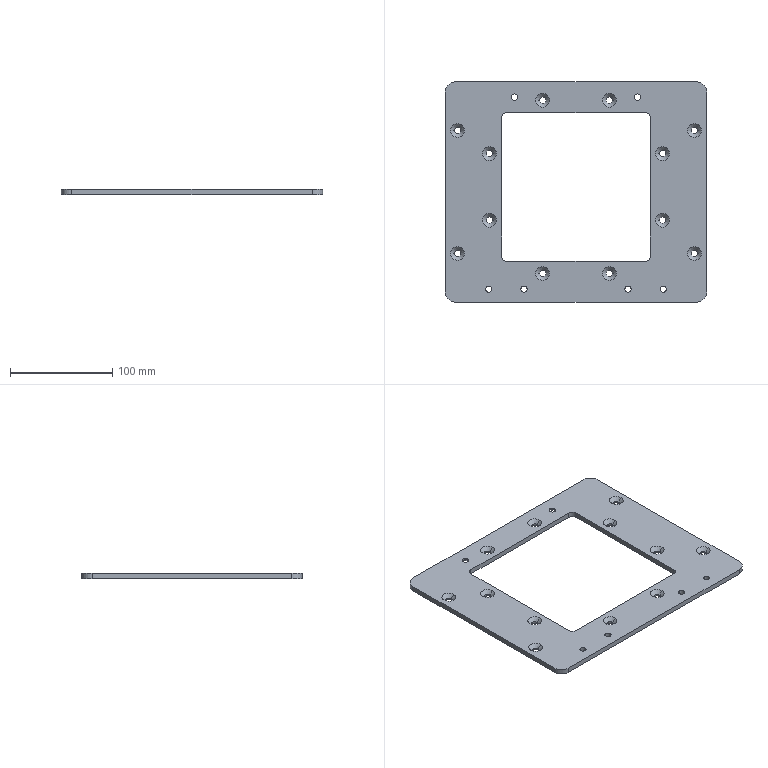NC program | NX | posted with a generic post | part box 255 x 215 x 5 mm
Whole program:
N10 G17 G21 G94 G90
(PLANAR_MILL_COPY_COPY_COPY_COPY_COPY , TOOL : D6A45)
N12 T01 M6
N14 G54
N16 G17 G0 G90 X-0.866 Y109.4 S9500 M3
N18 G43 Z30. H1
N20 Z0.
N22 G94 G1 Z-1.5 F1250.
N24 G3 X0. Y108.9 R1.
N26 G1 X117.5
N28 G2 X128.9 Y97.5 R11.4
N30 G1 Y-97.5
N32 G2 X117.5 Y-108.9 R11.4
N34 G1 X-117.5
N36 G2 X-128.9 Y-97.5 R11.4
N38 G1 Y97.5
N40 G2 X-117.5 Y108.9 R11.4
N42 G1 X0.
N44 G3 X0.866 Y109.4 R1.
N46 G1 Z0.
N48 G0 Z30.
N50 Y75.6
N52 Z0.
N54 G1 Z-1.5
N56 G3 X0. Y76.1 R1.
N58 G1 X-67.5
N60 G3 X-71.1 Y72.5 R3.6
N62 G1 Y-62.5
N64 G3 X-67.5 Y-66.1 R3.6
N66 G1 X67.5
N68 G3 X71.1 Y-62.5 R3.6
N70 G1 Y72.5
N72 G3 X67.5 Y76.1 R3.6
N74 G1 X0.
N76 G3 X-0.866 Y75.6 R1.
N78 G1 Z0.
N80 G0 Z30.
N82 X-31.634 Y90.85
N84 Z0.
N86 G1 Z-1.5
N88 G3 X-32.5 Y91.35 R1.
N90 X-34.35 Y89.5 R1.85
N92 X-32.5 Y91.35 R-1.85
N94 X-33.366 Y90.85 R1.
N96 G1 Z0.
N98 G0 Z30.
N100 X33.366
N102 Z0.
N104 G1 Z-1.5
N106 G3 X32.5 Y91.35 R1.
N108 X30.65 Y89.5 R1.85
N110 X32.5 Y91.35 R-1.85
N112 X31.634 Y90.85 R1.
N114 G1 Z0.
N116 G0 Z30.
N118 X116.85 Y59.134
N120 Z0.
N122 G1 Z-1.5
N124 G3 X117.35 Y60. R1.
N126 X115.5 Y61.85 R1.85
N128 X117.35 Y60. R-1.85
N130 X116.85 Y60.866 R1.
N132 G1 Z0.
N134 G0 Z30.
N136 X85.85 Y36.634
N138 Z0.
N140 G1 Z-1.5
N142 G3 X86.35 Y37.5 R1.
N144 X84.5 Y39.35 R1.85
N146 X86.35 Y37.5 R-1.85
N148 X85.85 Y38.366 R1.
N150 G1 Z0.
N152 G0 Z30.
N154 Y-28.366
N156 Z0.
N158 G1 Z-1.5
N160 G3 X86.35 Y-27.5 R1.
N162 X84.5 Y-25.65 R1.85
N164 X86.35 Y-27.5 R-1.85
N166 X85.85 Y-26.634 R1.
N168 G1 Z0.
N170 G0 Z30.
N172 X116.85 Y-60.866
N174 Z0.
N176 G1 Z-1.5
N178 G3 X117.35 Y-60. R1.
N180 X115.5 Y-58.15 R1.85
N182 X117.35 Y-60. R-1.85
N184 X116.85 Y-59.134 R1.
N186 G1 Z0.
N188 G0 Z30.
N190 X84.384 Y-95.95
N192 Z0.
N194 G1 Z-1.5
N196 G3 X85.25 Y-96.45 R1.
N198 X86.85 Y-94.85 R1.6
N200 X85.25 Y-96.45 R-1.6
N202 X86.116 Y-95.95 R1.
N204 G1 Z0.
N206 G0 Z30.
N208 X49.884
N210 Z0.
N212 G1 Z-1.5
N214 G3 X50.75 Y-96.45 R1.
N216 X52.35 Y-94.85 R1.6
N218 X50.75 Y-96.45 R-1.6
N220 X51.616 Y-95.95 R1.
N222 G1 Z0.
N224 G0 Z30.
N226 X31.634 Y-80.85
N228 Z0.
N230 G1 Z-1.5
N232 G3 X32.5 Y-81.35 R1.
N234 X34.35 Y-79.5 R1.85
N236 X32.5 Y-81.35 R-1.85
N238 X33.366 Y-80.85 R1.
N240 G1 Z0.
N242 G0 Z30.
N244 X-33.366
N246 Z0.
N248 G1 Z-1.5
N250 G3 X-32.5 Y-81.35 R1.
N252 X-30.65 Y-79.5 R1.85
N254 X-32.5 Y-81.35 R-1.85
N256 X-31.634 Y-80.85 R1.
N258 G1 Z0.
N260 G0 Z30.
N262 X-51.616 Y-95.95
N264 Z0.
N266 G1 Z-1.5
N268 G3 X-50.75 Y-96.45 R1.
N270 X-49.15 Y-94.85 R1.6
N272 X-50.75 Y-96.45 R-1.6
N274 X-49.884 Y-95.95 R1.
N276 G1 Z0.
N278 G0 Z30.
N280 X-86.116
N282 Z0.
N284 G1 Z-1.5
N286 G3 X-85.25 Y-96.45 R1.
N288 X-83.65 Y-94.85 R1.6
N290 X-85.25 Y-96.45 R-1.6
N292 X-84.384 Y-95.95 R1.
N294 G1 Z0.
N296 G0 Z30.
N298 X-116.85 Y-59.134
N300 Z0.
N302 G1 Z-1.5
N304 G3 X-117.35 Y-60. R1.
N306 X-115.5 Y-61.85 R1.85
N308 X-117.35 Y-60. R-1.85
N310 X-116.85 Y-60.866 R1.
N312 G1 Z0.
N314 G0 Z30.
N316 X-85.85 Y-26.634
N318 Z0.
N320 G1 Z-1.5
N322 G3 X-86.35 Y-27.5 R1.
N324 X-84.5 Y-29.35 R1.85
N326 X-86.35 Y-27.5 R-1.85
N328 X-85.85 Y-28.366 R1.
N330 G1 Z0.
N332 G0 Z30.
N334 Y38.366
N336 Z0.
N338 G1 Z-1.5
N340 G3 X-86.35 Y37.5 R1.
N342 X-84.5 Y35.65 R1.85
N344 X-86.35 Y37.5 R-1.85
N346 X-85.85 Y36.634 R1.
N348 G1 Z0.
N350 G0 Z30.
N352 X-116.85 Y60.866
N354 Z0.
N356 G1 Z-1.5
N358 G3 X-117.35 Y60. R1.
N360 X-115.5 Y58.15 R1.85
N362 X-117.35 Y60. R-1.85
N364 X-116.85 Y59.134 R1.
N366 G1 Z0.
N368 G0 Z30.
(ZLEVEL_PROFILE_COPY_1_COPY_1_COPY , TOOL : D6A45)
N370 X-59.025 Y98.532
N372 Z1.5
N374 G1 X-59.393 Y98.621 Z1.48 F1000.
N376 X-60.606 Z1.417
N378 X-61.54 Y98.455 Z1.367
N380 X-62.438 Y98.147 Z1.317
N382 X-63.499 Y97.558 Z1.254
N384 X-64.726 Y96.437 Z1.166
N386 X-65.607 Y95.028 Z1.079
N388 X-66.079 Y93.435 Z0.992
N390 X-66.108 Y91.774 Z0.905
N392 X-65.69 Y90.165 Z0.818
N394 X-64.858 Y88.727 Z0.731
N396 X-63.671 Y87.564 Z0.644
N398 X-62.63 Y86.94 Z0.58
N400 X-61.046 Y86.438 Z0.493
N402 X-59.385 Y86.38 Z0.406
N404 X-57.769 Y86.767 Z0.319
N406 X-56.316 Y87.573 Z0.232
N408 X-55.132 Y88.739 Z0.145
N410 X-54.303 Y90.179 Z0.058
N412 X-53.89 Y91.788 Z-0.029
N414 X-53.869 Y93.002 Z-0.093
N416 X-54.242 Y94.665 Z-0.182
N418 X-55.057 Y96.163 Z-0.272
N420 X-56.253 Y97.378 Z-0.361
N422 X-57.736 Y98.22 Z-0.45
N424 X-59.393 Y98.621 Z-0.54
N426 X-59.999 Z-0.571
N428 G3 X-66.121 Y92.5 R6.121 F1500.
N430 X-59.999 Y98.621 R-6.121
N432 G1 X-60.513 Y98.577 Z-0.579
N434 X-61.025 Y98.518 Z-0.588
N436 X-61.521 Y98.383 Z-0.596
N438 X-62.016 Y98.245 Z-0.604
N440 X-62.418 Y98.067 Z-0.61
N442 X-62.818 Y97.882 Z-0.617
N444 X-62.945 Y97.81 Z-0.62
N446 X-63.422 Y97.486 Z-0.629
N448 X-63.885 Y97.143 Z-0.638
N450 X-64.32 Y96.722 Z-0.647
N452 X-64.68 Y96.312 Z-0.656
N454 X-65.049 Y95.783 Z-0.666
N456 X-65.301 Y95.349 Z-0.673
N458 X-65.566 Y94.755 Z-0.684
N460 X-65.727 Y94.289 Z-0.691
N462 X-65.878 Y93.653 Z-0.701
N464 X-65.945 Y93.171 Z-0.709
N466 X-65.968 Y92.728 Z-0.716
N468 X-65.976 Y92.506 Z-0.719
N470 X-65.967 Y92.349 Z-0.722
N472 X-65.946 Y92.035 Z-0.727
N474 X-65.853 Y91.477 Z-0.736
N476 X-65.734 Y90.923 Z-0.745
N478 X-65.534 Y90.356 Z-0.754
N480 X-65.315 Y89.874 Z-0.762
N482 X-64.989 Y89.32 Z-0.772
N484 X-64.708 Y88.926 Z-0.78
N486 X-64.295 Y88.456 Z-0.79
N488 X-63.935 Y88.112 Z-0.797
N490 X-63.546 Y87.817 Z-0.805
N492 X-63.147 Y87.535 Z-0.813
N494 X-63.024 Y87.462 Z-0.815
N496 X-62.523 Y87.218 Z-0.824
N498 X-62.01 Y86.997 Z-0.832
N500 X-61.439 Y86.833 Z-0.842
N502 X-60.93 Y86.733 Z-0.85
N504 X-60.299 Y86.68 Z-0.859
N506 X-59.822 Y86.679 Z-0.867
N508 X-59.193 Y86.746 Z-0.877
N510 X-58.727 Y86.835 Z-0.884
N512 X-58.123 Y87.017 Z-0.894
N514 X-57.685 Y87.194 Z-0.901
N516 X-57.305 Y87.386 Z-0.908
N518 X-57.117 Y87.487 Z-0.911
N520 X-56.989 Y87.572 Z-0.914
N522 X-56.733 Y87.742 Z-0.919
N524 X-56.217 Y88.151 Z-0.929
N526 X-55.904 Y88.458 Z-0.936
N528 X-55.481 Y88.955 Z-0.946
N530 X-55.227 Y89.316 Z-0.953
N532 X-54.916 Y89.868 Z-0.963
N534 X-54.726 Y90.283 Z-0.97
N536 X-54.53 Y90.859 Z-0.979
N538 X-54.419 Y91.325 Z-0.987
N540 X-54.36 Y91.794 Z-0.994
N542 X-54.316 Y92.266 Z-1.002
N544 X-54.314 Y92.403 Z-1.004
N546 X-54.346 Y92.902 Z-1.012
N548 X-54.401 Y93.399 Z-1.019
N550 X-54.521 Y93.922 Z-1.028
N552 X-54.661 Y94.363 Z-1.035
N554 X-54.864 Y94.817 Z-1.043
N556 X-55.084 Y95.264 Z-1.051
N558 X-55.366 Y95.706 Z-1.059
N560 X-55.657 Y96.074 Z-1.066
N562 X-56.005 Y96.426 Z-1.074
N564 X-56.362 Y96.768 Z-1.081
N566 X-56.773 Y97.077 Z-1.089
N568 X-57.176 Y97.327 Z-1.097
N570 X-57.619 Y97.541 Z-1.105
N572 X-58.072 Y97.734 Z-1.112
N574 X-58.577 Y97.883 Z-1.12
N576 X-59.023 Y97.976 Z-1.128
N578 X-59.511 Y98.02 Z-1.135
N580 X-59.999 Y98.047 Z-1.143
N582 X-60.637 Y97.999 Z-1.154
N584 X-60.885 Y97.96 Z-1.158
N586 X-61.315 Y97.85 Z-1.166
N588 X-61.743 Y97.733 Z-1.174
N590 X-62.183 Y97.561 Z-1.182
N592 X-62.551 Y97.373 Z-1.189
N594 X-62.989 Y97.089 Z-1.198
N596 X-63.416 Y96.788 Z-1.207
N598 X-63.819 Y96.416 Z-1.217
N600 X-64.152 Y96.053 Z-1.225
N602 X-64.502 Y95.579 Z-1.235
N604 X-64.734 Y95.194 Z-1.243
N606 X-64.995 Y94.652 Z-1.253
N608 X-65.141 Y94.243 Z-1.261
N610 X-65.25 Y93.849 Z-1.268
N612 X-65.3 Y93.651 Z-1.272
N614 X-65.321 Y93.513 Z-1.274
N616 X-65.361 Y93.236 Z-1.279
N618 X-65.385 Y92.723 Z-1.288
N620 Y92.21 Z-1.297
N622 X-65.318 Y91.669 Z-1.306
N624 X-65.216 Y91.2 Z-1.314
N626 X-65.033 Y90.647 Z-1.324
N628 X-64.86 Y90.244 Z-1.332
N630 X-64.574 Y89.732 Z-1.342
N632 X-64.331 Y89.375 Z-1.35
N634 X-63.954 Y88.923 Z-1.36
N636 X-63.649 Y88.624 Z-1.367
N638 X-63.187 Y88.244 Z-1.378
N640 X-62.84 Y88.019 Z-1.385
N642 X-62.302 Y87.731 Z-1.395
N644 X-61.934 Y87.578 Z-1.402
N646 X-61.367 Y87.405 Z-1.412
N648 X-60.965 Y87.318 Z-1.42
N650 X-60.391 Y87.256 Z-1.43
N652 X-59.967 Y87.246 Z-1.437
N654 X-59.394 Y87.291 Z-1.447
N656 X-58.976 Y87.364 Z-1.454
N658 X-58.413 Y87.515 Z-1.464
N660 X-58.029 Y87.667 Z-1.471
N662 X-57.491 Y87.933 Z-1.482
N664 X-57.159 Y88.141 Z-1.489
N666 X-56.692 Y88.5 Z-1.499
N668 X-56.398 Y88.77 Z-1.506
N670 X-56.018 Y89.197 Z-1.516
N672 X-55.771 Y89.529 Z-1.523
N674 X-55.479 Y90.014 Z-1.533
N676 X-55.3 Y90.39 Z-1.54
N678 X-55.101 Y90.926 Z-1.55
N680 X-55.002 Y91.321 Z-1.557
N682 X-54.907 Y91.909 Z-1.567
N684 X-54.886 Y92.289 Z-1.574
N686 X-54.892 Y92.706 Z-1.581
N688 X-54.904 Y92.914 Z-1.584
N690 X-54.924 Y93.047 Z-1.587
N692 X-54.965 Y93.314 Z-1.591
N694 X-55.114 Y93.932 Z-1.602
N696 X-55.246 Y94.299 Z-1.609
N698 X-55.508 Y94.856 Z-1.62
N700 X-55.717 Y95.205 Z-1.627
N702 X-56.076 Y95.685 Z-1.637
N704 X-56.358 Y95.995 Z-1.644
N706 X-56.798 Y96.387 Z-1.655
N708 X-57.141 Y96.639 Z-1.662
N710 X-57.646 Y96.932 Z-1.672
N712 X-58.034 Y97.111 Z-1.679
N714 X-58.584 Y97.297 Z-1.69
N716 X-59. Y97.394 Z-1.697
N718 X-59.498 Y97.452 Z-1.706
N720 X-60. Y97.478 Z-1.714
N722 X-60.572 Y97.436 Z-1.725
N724 X-61.141 Y97.322 Z-1.737
N726 X-61.579 Y97.191 Z-1.746
N728 X-62.12 Y96.956 Z-1.757
N730 X-62.51 Y96.743 Z-1.766
N732 X-62.986 Y96.403 Z-1.777
N734 X-63.324 Y96.114 Z-1.786
N736 X-63.696 Y95.714 Z-1.796
N738 X-63.988 Y95.333 Z-1.805
N740 X-64.328 Y94.744 Z-1.819
N742 X-64.473 Y94.435 Z-1.825
N744 X-64.658 Y93.874 Z-1.837
N746 X-64.758 Y93.459 Z-1.845
N748 X-64.824 Y92.883 Z-1.856
N750 X-64.836 Y92.449 Z-1.865
N752 X-64.779 Y91.895 Z-1.875
N754 X-64.697 Y91.449 Z-1.884
N756 X-64.526 Y90.91 Z-1.895
N758 X-64.359 Y90.504 Z-1.904
N760 X-64.08 Y90.014 Z-1.915
N762 X-63.833 Y89.652 Z-1.923
N764 X-63.463 Y89.236 Z-1.934
N766 X-63.145 Y88.932 Z-1.943
N768 X-62.695 Y88.602 Z-1.953
N770 X-62.325 Y88.372 Z-1.962
N772 X-61.823 Y88.146 Z-1.972
N774 X-61.411 Y87.997 Z-1.981
N776 X-60.915 Y87.887 Z-1.991
N778 X-60.442 Y87.82 Z-2.
N780 X-59.788 Y87.819 Z-2.013
N782 X-59.461 Y87.849 Z-2.019
N784 X-58.901 Y87.969 Z-2.03
N786 X-58.512 Y88.079 Z-2.038
N788 X-58.021 Y88.297 Z-2.049
N790 X-57.634 Y88.501 Z-2.057
N792 X-57.203 Y88.814 Z-2.067
N794 X-56.867 Y89.094 Z-2.076
N796 X-56.513 Y89.487 Z-2.086
N798 X-56.242 Y89.83 Z-2.095
N800 X-55.983 Y90.277 Z-2.105
N802 X-55.785 Y90.677 Z-2.113
N804 X-55.63 Y91.151 Z-2.123
N806 X-55.523 Y91.544 Z-2.131
N808 X-55.466 Y92.014 Z-2.14
N810 X-55.442 Y92.443 Z-2.148
N812 X-55.48 Y92.946 Z-2.158
N814 X-55.535 Y93.337 Z-2.166
N816 X-55.668 Y93.804 Z-2.175
N818 X-55.805 Y94.192 Z-2.183
N820 X-56.029 Y94.626 Z-2.192
N822 X-56.235 Y94.973 Z-2.2
N824 X-56.538 Y95.352 Z-2.21
N826 X-56.807 Y95.653 Z-2.218
N828 X-57.175 Y95.961 Z-2.227
N830 X-57.499 Y96.205 Z-2.235
N832 X-57.916 Y96.432 Z-2.244
N834 X-58.282 Y96.61 Z-2.252
N836 X-58.749 Y96.753 Z-2.261
N838 X-59.127 Y96.852 Z-2.269
N840 X-59.561 Y96.904 Z-2.277
N842 X-60. Y96.909 Z-2.286
N844 X-60.626 Y96.85 Z-2.3
N846 X-60.953 Y96.794 Z-2.307
N848 X-61.453 Y96.629 Z-2.318
N850 X-61.852 Y96.466 Z-2.328
N852 X-62.3 Y96.199 Z-2.339
N854 X-62.655 Y95.953 Z-2.349
N856 X-62.995 Y95.636 Z-2.359
N858 X-63.325 Y95.283 Z-2.37
N860 X-63.492 Y95.062 Z-2.376
N862 X-63.642 Y94.83 Z-2.382
N864 X-63.741 Y94.661 Z-2.386
N866 X-63.831 Y94.486 Z-2.39
N868 X-64.06 Y93.897 Z-2.404
N870 X-64.166 Y93.544 Z-2.412
N872 X-64.248 Y92.982 Z-2.425
N874 X-64.277 Y92.555 Z-2.434
N876 X-64.226 Y92.017 Z-2.446
N878 X-64.151 Y91.573 Z-2.456
N880 X-63.976 Y91.063 Z-2.468
N882 X-63.805 Y90.65 Z-2.478
N884 X-63.525 Y90.201 Z-2.489
N886 X-63.261 Y89.835 Z-2.499
N888 X-62.884 Y89.458 Z-2.511
N890 X-62.547 Y89.169 Z-2.521
N892 X-62.092 Y88.891 Z-2.533
N894 X-61.702 Y88.69 Z-2.542
N896 X-61.255 Y88.542 Z-2.553
N898 X-60.773 Y88.423 Z-2.564
N900 X-60.482 Y88.387 Z-2.57
N902 X-60.188 Y88.368 Z-2.577
N904 X-60.001 Y88.37 Z-2.581
N906 X-59.813 Y88.376 Z-2.585
N908 X-59.241 Y88.459 Z-2.598
N910 X-58.872 Y88.549 Z-2.606
N912 X-58.358 Y88.747 Z-2.618
N914 X-58. Y88.93 Z-2.627
N916 X-57.56 Y89.238 Z-2.639
N918 X-57.245 Y89.503 Z-2.648
N920 X-56.894 Y89.897 Z-2.659
N922 X-56.646 Y90.231 Z-2.669
N924 X-56.392 Y90.696 Z-2.68
N926 X-56.231 Y91.073 Z-2.689
N928 X-56.089 Y91.583 Z-2.701
N930 X-56.023 Y91.983 Z-2.71
N932 X-56.003 Y92.34 Z-2.718
N934 X-55.996 Y92.518 Z-2.722
N936 X-56.004 Y92.65 Z-2.724
N938 X-56.03 Y92.912 Z-2.73
N940 X-56.132 Y93.429 Z-2.742
N942 X-56.25 Y93.81 Z-2.751
N944 X-56.363 Y94.068 Z-2.757
N946 X-56.484 Y94.322 Z-2.763
N948 X-56.67 Y94.629 Z-2.771
N950 X-56.947 Y94.993 Z-2.781
N952 X-57.172 Y95.238 Z-2.788
N954 X-57.513 Y95.537 Z-2.798
N956 X-57.782 Y95.733 Z-2.806
N958 X-58.173 Y95.957 Z-2.816
N960 X-58.477 Y96.095 Z-2.823
N962 X-58.903 Y96.236 Z-2.833
N964 X-59.226 Y96.31 Z-2.84
N966 X-60. Y96.372 Z-2.857
N968 X-60.475 Y96.332 Z-2.869
N970 X-60.766 Y96.276 Z-2.877
N972 X-61.211 Y96.15 Z-2.888
N974 X-61.495 Y96.031 Z-2.896
N976 X-61.913 Y95.817 Z-2.908
N978 X-62.157 Y95.647 Z-2.916
N980 X-62.534 Y95.348 Z-2.928
N982 X-62.727 Y95.142 Z-2.935
N984 X-63.051 Y94.754 Z-2.948
N986 X-63.183 Y94.536 Z-2.954
N988 X-63.368 Y94.204 Z-2.964
N990 X-63.449 Y94.033 Z-2.969
N992 X-63.484 Y93.936 Z-2.971
N994 X-63.546 Y93.74 Z-2.976
N996 X-63.654 Y93.318 Z-2.987
N998 X-63.731 Y92.889 Z-2.998
N1000 X-63.722 Y92.692 Z-3.003
N1002 X-63.742 Y92.497 Z-3.008
N1004 X-63.728 Y92.263 Z-3.014
N1006 X-63.699 Y92.02 Z-3.02
N1008 X-63.585 Y91.519 Z-3.033
N1010 X-63.468 Y91.188 Z-3.042
N1012 X-63.308 Y90.846 Z-3.052
N1014 X-63.084 Y90.479 Z-3.063
N1016 X-63.054 Y90.436 Z-3.064
N1018 X-62.696 Y90.007 Z-3.078
N1020 X-62.481 Y89.803 Z-3.086
N1022 X-62.076 Y89.496 Z-3.098
N1024 X-61.782 Y89.322 Z-3.107
N1026 X-61.328 Y89.121 Z-3.12
N1028 X-60.995 Y89.018 Z-3.128
N1030 X-60.511 Y88.927 Z-3.141
N1032 X-60.164 Y88.903 Z-3.15
N1034 X-59.676 Y88.927 Z-3.162
N1036 X-59.334 Y88.983 Z-3.171
N1038 X-58.867 Y89.118 Z-3.183
N1040 X-58.55 Y89.251 Z-3.192
N1042 X-58.129 Y89.488 Z-3.204
N1044 X-57.852 Y89.689 Z-3.213
N1046 X-57.538 Y89.975 Z-3.223
N1048 X-57.278 Y90.274 Z-3.233
N1050 X-57.154 Y90.443 Z-3.239
N1052 X-57.041 Y90.62 Z-3.244
N1054 X-56.944 Y90.792 Z-3.249
N1056 X-56.856 Y90.971 Z-3.254
N1058 X-56.682 Y91.439 Z-3.267
N1060 X-56.608 Y91.741 Z-3.275
N1062 X-56.549 Y92.214 Z-3.287
N1064 X-56.545 Y92.544 Z-3.295
N1066 X-56.595 Y93.011 Z-3.307
N1068 X-56.668 Y93.334 Z-3.315
N1070 X-56.821 Y93.769 Z-3.327
N1072 X-56.968 Y94.071 Z-3.335
N1074 X-57.2 Y94.435 Z-3.346
N1076 X-57.395 Y94.679 Z-3.354
N1078 X-57.701 Y94.984 Z-3.365
N1080 X-57.941 Y95.177 Z-3.373
N1082 X-58.249 Y95.377 Z-3.382
N1084 X-58.578 Y95.543 Z-3.392
N1086 X-58.689 Y95.589 Z-3.395
N1088 X-58.801 Y95.631 Z-3.398
N1090 X-59.036 Y95.704 Z-3.404
N1092 X-59.276 Y95.76 Z-3.41
N1094 X-59.635 Y95.811 Z-3.419
N1096 X-60. Y95.821 Z-3.429
N1098 X-60.33 Y95.795 Z-3.438
N1100 X-60.492 Y95.77 Z-3.443
N1102 X-60.613 Y95.745 Z-3.447
N1104 X-60.849 Y95.668 Z-3.455
N1106 X-61.433 Y95.447 Z-3.473
N1108 X-61.629 Y95.32 Z-3.48
N1110 X-62.107 Y94.978 Z-3.498
N1112 X-62.284 Y94.782 Z-3.506
N1114 X-62.555 Y94.478 Z-3.518
N1116 X-62.669 Y94.312 Z-3.524
N1118 X-62.709 Y94.244 Z-3.527
N1120 X-62.779 Y94.102 Z-3.531
N1122 X-63.013 Y93.575 Z-3.549
N1124 X-63.071 Y93.321 Z-3.557
N1126 X-63.118 Y93.031 Z-3.565
N1128 X-63.153 Y92.74 Z-3.574
N1130 X-63.159 Y92.497 Z-3.582
N1132 X-63.138 Y92.161 Z-3.592
N1134 X-63.085 Y91.909 Z-3.6
N1136 X-62.999 Y91.628 Z-3.608
N1138 X-62.899 Y91.35 Z-3.617
N1140 X-62.76 Y91.043 Z-3.628
N1142 X-62.617 Y90.837 Z-3.635
N1144 X-62.404 Y90.544 Z-3.646
N1146 X-62.286 Y90.409 Z-3.651
N1148 X-62.229 Y90.354 Z-3.654
N1150 X-62.109 Y90.253 Z-3.659
N1152 X-61.83 Y90.024 Z-3.669
N1154 X-61.612 Y89.89 Z-3.677
N1156 X-61.471 Y89.822 Z-3.682
N1158 X-60.971 Y89.609 Z-3.698
N1160 X-60.754 Y89.564 Z-3.705
N1162 X-60.219 Y89.48 Z-3.721
N1164 X-60. Y89.488 Z-3.728
N1166 X-59.677 Y89.508 Z-3.738
N1168 X-59.431 Y89.552 Z-3.745
N1170 X-59.258 Y89.607 Z-3.751
N1172 X-58.982 Y89.705 Z-3.759
N1174 X-58.715 Y89.824 Z-3.768
N1176 X-58.572 Y89.901 Z-3.773
N1178 X-58.318 Y90.061 Z-3.782
N1180 X-58.198 Y90.15 Z-3.787
N1182 X-58.123 Y90.213 Z-3.79
N1184 X-57.986 Y90.354 Z-3.796
N1186 X-57.659 Y90.729 Z-3.811
N1188 X-57.534 Y90.933 Z-3.818
N1190 X-57.412 Y91.178 Z-3.826
N1192 X-57.302 Y91.429 Z-3.834
N1194 X-57.205 Y91.715 Z-3.843
N1196 X-57.162 Y91.955 Z-3.851
N1198 X-57.124 Y92.313 Z-3.862
N1200 X-57.125 Y92.495 Z-3.867
N1202 X-57.141 Y92.777 Z-3.876
N1204 X-57.179 Y93.004 Z-3.883
N1206 X-57.231 Y93.176 Z-3.888
N1208 X-57.397 Y93.649 Z-3.903
N1210 X-57.489 Y93.811 Z-3.909
N1212 X-57.746 Y94.198 Z-3.923
N1214 X-57.889 Y94.36 Z-3.929
N1216 X-58.185 Y94.64 Z-3.941
N1218 X-58.409 Y94.791 Z-3.95
N1220 X-58.777 Y95. Z-3.962
N1222 X-59.009 Y95.09 Z-3.97
N1224 X-59.499 Y95.208 Z-3.985
N1226 X-59.749 Y95.23 Z-3.992
N1228 X-60. Y95.243 Z-4.
N1230 G3 X-62.743 Y92.5 R2.743
N1232 X-60. Y95.243 R-2.743
N1234 G1 Z-2.5
N1236 G0 Z30.
N1238 X60.975 Y98.532
N1240 Z1.5
N1242 G1 X60.607 Y98.621 Z1.48 F1000.
N1244 X59.394 Z1.417
N1246 X58.46 Y98.455 Z1.367
N1248 X57.562 Y98.147 Z1.317
N1250 X56.501 Y97.558 Z1.254
N1252 X55.274 Y96.437 Z1.166
N1254 X54.393 Y95.028 Z1.079
N1256 X53.921 Y93.435 Z0.992
N1258 X53.892 Y91.774 Z0.905
N1260 X54.31 Y90.165 Z0.818
N1262 X55.142 Y88.727 Z0.731
N1264 X56.329 Y87.564 Z0.644
N1266 X57.37 Y86.94 Z0.58
N1268 X58.954 Y86.438 Z0.493
N1270 X60.615 Y86.38 Z0.406
N1272 X62.231 Y86.767 Z0.319
N1274 X63.684 Y87.573 Z0.232
N1276 X64.868 Y88.739 Z0.145
N1278 X65.697 Y90.179 Z0.058
N1280 X66.11 Y91.788 Z-0.029
N1282 X66.131 Y93.002 Z-0.093
N1284 X65.758 Y94.665 Z-0.182
N1286 X64.943 Y96.163 Z-0.272
N1288 X63.747 Y97.378 Z-0.361
N1290 X62.264 Y98.22 Z-0.45
N1292 X60.607 Y98.621 Z-0.54
N1294 X60.001 Z-0.571
N1296 G3 X53.879 Y92.5 R6.121 F1500.
N1298 X60.001 Y98.621 R-6.121
N1300 G1 X59.487 Y98.577 Z-0.579
N1302 X58.975 Y98.518 Z-0.588
N1304 X58.479 Y98.383 Z-0.596
N1306 X57.984 Y98.245 Z-0.604
N1308 X57.582 Y98.067 Z-0.61
N1310 X57.182 Y97.882 Z-0.617
N1312 X57.055 Y97.81 Z-0.62
N1314 X56.578 Y97.486 Z-0.629
N1316 X56.115 Y97.143 Z-0.638
N1318 X55.68 Y96.722 Z-0.647
N1320 X55.32 Y96.312 Z-0.656
N1322 X54.951 Y95.783 Z-0.666
N1324 X54.699 Y95.349 Z-0.673
N1326 X54.434 Y94.755 Z-0.684
N1328 X54.273 Y94.289 Z-0.691
N1330 X54.122 Y93.653 Z-0.701
N1332 X54.055 Y93.171 Z-0.709
N1334 X54.032 Y92.728 Z-0.716
N1336 X54.024 Y92.506 Z-0.719
N1338 X54.033 Y92.349 Z-0.722
N1340 X54.054 Y92.035 Z-0.727
N1342 X54.147 Y91.477 Z-0.736
N1344 X54.266 Y90.923 Z-0.745
N1346 X54.466 Y90.356 Z-0.754
N1348 X54.685 Y89.874 Z-0.762
N1350 X55.011 Y89.32 Z-0.772
N1352 X55.292 Y88.926 Z-0.78
N1354 X55.705 Y88.456 Z-0.79
N1356 X56.065 Y88.112 Z-0.797
N1358 X56.454 Y87.817 Z-0.805
N1360 X56.853 Y87.535 Z-0.813
N1362 X56.976 Y87.462 Z-0.815
N1364 X57.477 Y87.218 Z-0.824
N1366 X57.99 Y86.997 Z-0.832
N1368 X58.561 Y86.833 Z-0.842
N1370 X59.07 Y86.733 Z-0.85
N1372 X59.701 Y86.68 Z-0.859
N1374 X60.178 Y86.679 Z-0.867
N1376 X60.807 Y86.746 Z-0.877
N1378 X61.273 Y86.835 Z-0.884
N1380 X61.877 Y87.017 Z-0.894
N1382 X62.315 Y87.194 Z-0.901
N1384 X62.695 Y87.386 Z-0.908
N1386 X62.883 Y87.487 Z-0.911
N1388 X63.011 Y87.572 Z-0.914
N1390 X63.267 Y87.742 Z-0.919
N1392 X63.783 Y88.151 Z-0.929
N1394 X64.096 Y88.458 Z-0.936
N1396 X64.519 Y88.955 Z-0.946
N1398 X64.773 Y89.316 Z-0.953
N1400 X65.084 Y89.868 Z-0.963
N1402 X65.274 Y90.283 Z-0.97
N1404 X65.47 Y90.859 Z-0.979
N1406 X65.581 Y91.325 Z-0.987
N1408 X65.64 Y91.794 Z-0.994
N1410 X65.684 Y92.266 Z-1.002
N1412 X65.686 Y92.403 Z-1.004
N1414 X65.654 Y92.902 Z-1.012
N1416 X65.599 Y93.399 Z-1.019
N1418 X65.479 Y93.922 Z-1.028
N1420 X65.339 Y94.363 Z-1.035
N1422 X65.136 Y94.817 Z-1.043
N1424 X64.916 Y95.264 Z-1.051
N1426 X64.634 Y95.706 Z-1.059
N1428 X64.343 Y96.074 Z-1.066
N1430 X63.995 Y96.426 Z-1.074
N1432 X63.638 Y96.768 Z-1.081
N1434 X63.227 Y97.077 Z-1.089
N1436 X62.824 Y97.327 Z-1.097
N1438 X62.381 Y97.541 Z-1.105
N1440 X61.928 Y97.734 Z-1.112
N1442 X61.423 Y97.883 Z-1.12
N1444 X60.977 Y97.976 Z-1.128
N1446 X60.489 Y98.02 Z-1.135
N1448 X60.001 Y98.047 Z-1.143
N1450 X59.363 Y97.999 Z-1.154
N1452 X59.115 Y97.96 Z-1.158
N1454 X58.685 Y97.85 Z-1.166
N1456 X58.257 Y97.733 Z-1.174
N1458 X57.817 Y97.561 Z-1.182
N1460 X57.449 Y97.373 Z-1.189
N1462 X57.011 Y97.089 Z-1.198
N1464 X56.584 Y96.788 Z-1.207
N1466 X56.181 Y96.416 Z-1.217
N1468 X55.848 Y96.053 Z-1.225
N1470 X55.498 Y95.579 Z-1.235
N1472 X55.266 Y95.194 Z-1.243
N1474 X55.005 Y94.652 Z-1.253
N1476 X54.859 Y94.243 Z-1.261
N1478 X54.75 Y93.849 Z-1.268
N1480 X54.7 Y93.651 Z-1.272
N1482 X54.679 Y93.513 Z-1.274
N1484 X54.639 Y93.236 Z-1.279
N1486 X54.615 Y92.723 Z-1.288
N1488 Y92.21 Z-1.297
N1490 X54.682 Y91.669 Z-1.306
N1492 X54.784 Y91.2 Z-1.314
N1494 X54.967 Y90.647 Z-1.324
N1496 X55.14 Y90.244 Z-1.332
N1498 X55.426 Y89.732 Z-1.342
N1500 X55.669 Y89.375 Z-1.35
N1502 X56.046 Y88.923 Z-1.36
N1504 X56.351 Y88.624 Z-1.367
N1506 X56.813 Y88.244 Z-1.378
N1508 X57.16 Y88.019 Z-1.385
N1510 X57.698 Y87.731 Z-1.395
N1512 X58.066 Y87.578 Z-1.402
N1514 X58.633 Y87.405 Z-1.412
N1516 X59.035 Y87.318 Z-1.42
N1518 X59.609 Y87.256 Z-1.43
N1520 X60.033 Y87.246 Z-1.437
N1522 X60.606 Y87.291 Z-1.447
N1524 X61.024 Y87.364 Z-1.454
N1526 X61.587 Y87.515 Z-1.464
N1528 X61.971 Y87.667 Z-1.471
N1530 X62.509 Y87.933 Z-1.482
N1532 X62.841 Y88.141 Z-1.489
N1534 X63.308 Y88.5 Z-1.499
N1536 X63.602 Y88.77 Z-1.506
N1538 X63.982 Y89.197 Z-1.516
N1540 X64.229 Y89.529 Z-1.523
N1542 X64.521 Y90.014 Z-1.533
N1544 X64.7 Y90.39 Z-1.54
N1546 X64.899 Y90.926 Z-1.55
N1548 X64.998 Y91.321 Z-1.557
N1550 X65.093 Y91.909 Z-1.567
N1552 X65.114 Y92.289 Z-1.574
N1554 X65.108 Y92.706 Z-1.581
N1556 X65.096 Y92.914 Z-1.584
N1558 X65.076 Y93.047 Z-1.587
N1560 X65.035 Y93.314 Z-1.591
N1562 X64.886 Y93.932 Z-1.602
N1564 X64.754 Y94.299 Z-1.609
N1566 X64.492 Y94.856 Z-1.62
N1568 X64.283 Y95.205 Z-1.627
N1570 X63.924 Y95.685 Z-1.637
N1572 X63.642 Y95.995 Z-1.644
N1574 X63.202 Y96.387 Z-1.655
N1576 X62.859 Y96.639 Z-1.662
N1578 X62.354 Y96.932 Z-1.672
N1580 X61.966 Y97.111 Z-1.679
N1582 X61.416 Y97.297 Z-1.69
N1584 X61. Y97.394 Z-1.697
N1586 X60.502 Y97.452 Z-1.706
N1588 X60. Y97.478 Z-1.714
N1590 X59.428 Y97.436 Z-1.725
N1592 X58.859 Y97.322 Z-1.737
N1594 X58.421 Y97.191 Z-1.746
N1596 X57.88 Y96.956 Z-1.757
N1598 X57.49 Y96.743 Z-1.766
N1600 X57.014 Y96.403 Z-1.777
N1602 X56.676 Y96.114 Z-1.786
N1604 X56.304 Y95.714 Z-1.796
N1606 X56.012 Y95.333 Z-1.805
N1608 X55.672 Y94.744 Z-1.819
N1610 X55.527 Y94.435 Z-1.825
N1612 X55.342 Y93.874 Z-1.837
N1614 X55.242 Y93.459 Z-1.845
N1616 X55.176 Y92.883 Z-1.856
N1618 X55.164 Y92.449 Z-1.865
N1620 X55.221 Y91.895 Z-1.875
N1622 X55.303 Y91.449 Z-1.884
N1624 X55.474 Y90.91 Z-1.895
N1626 X55.641 Y90.504 Z-1.904
N1628 X55.92 Y90.014 Z-1.915
N1630 X56.167 Y89.652 Z-1.923
N1632 X56.537 Y89.236 Z-1.934
N1634 X56.855 Y88.932 Z-1.943
N1636 X57.305 Y88.602 Z-1.953
N1638 X57.675 Y88.372 Z-1.962
N1640 X58.177 Y88.146 Z-1.972
N1642 X58.589 Y87.997 Z-1.981
N1644 X59.085 Y87.887 Z-1.991
N1646 X59.558 Y87.82 Z-2.
N1648 X60.212 Y87.819 Z-2.013
N1650 X60.539 Y87.849 Z-2.019
N1652 X61.099 Y87.969 Z-2.03
N1654 X61.488 Y88.079 Z-2.038
N1656 X61.979 Y88.297 Z-2.049
N1658 X62.366 Y88.501 Z-2.057
N1660 X62.797 Y88.814 Z-2.067
N1662 X63.133 Y89.094 Z-2.076
N1664 X63.487 Y89.487 Z-2.086
N1666 X63.758 Y89.83 Z-2.095
N1668 X64.017 Y90.277 Z-2.105
N1670 X64.215 Y90.677 Z-2.113
N1672 X64.37 Y91.151 Z-2.123
N1674 X64.477 Y91.544 Z-2.131
N1676 X64.534 Y92.014 Z-2.14
N1678 X64.558 Y92.443 Z-2.148
N1680 X64.52 Y92.946 Z-2.158
N1682 X64.465 Y93.337 Z-2.166
N1684 X64.332 Y93.804 Z-2.175
N1686 X64.195 Y94.192 Z-2.183
N1688 X63.971 Y94.626 Z-2.192
N1690 X63.765 Y94.973 Z-2.2
N1692 X63.462 Y95.352 Z-2.21
N1694 X63.193 Y95.653 Z-2.218
N1696 X62.825 Y95.961 Z-2.227
N1698 X62.501 Y96.205 Z-2.235
N1700 X62.084 Y96.432 Z-2.244
N1702 X61.718 Y96.61 Z-2.252
N1704 X61.251 Y96.753 Z-2.261
N1706 X60.873 Y96.852 Z-2.269
N1708 X60.439 Y96.904 Z-2.277
N1710 X60. Y96.909 Z-2.286
N1712 X59.374 Y96.85 Z-2.3
N1714 X59.047 Y96.794 Z-2.307
N1716 X58.547 Y96.629 Z-2.318
N1718 X58.148 Y96.466 Z-2.328
N1720 X57.7 Y96.199 Z-2.339
N1722 X57.345 Y95.953 Z-2.349
N1724 X57.005 Y95.636 Z-2.359
N1726 X56.675 Y95.283 Z-2.37
N1728 X56.508 Y95.062 Z-2.376
N1730 X56.358 Y94.83 Z-2.382
N1732 X56.259 Y94.661 Z-2.386
N1734 X56.169 Y94.486 Z-2.39
N1736 X55.94 Y93.897 Z-2.404
N1738 X55.834 Y93.544 Z-2.412
N1740 X55.752 Y92.982 Z-2.425
N1742 X55.723 Y92.555 Z-2.434
N1744 X55.774 Y92.017 Z-2.446
N1746 X55.849 Y91.573 Z-2.456
N1748 X56.024 Y91.063 Z-2.468
N1750 X56.195 Y90.65 Z-2.478
N1752 X56.475 Y90.201 Z-2.489
N1754 X56.739 Y89.835 Z-2.499
N1756 X57.116 Y89.458 Z-2.511
N1758 X57.453 Y89.169 Z-2.521
N1760 X57.908 Y88.891 Z-2.533
N1762 X58.298 Y88.69 Z-2.542
N1764 X58.745 Y88.542 Z-2.553
N1766 X59.227 Y88.423 Z-2.564
N1768 X59.518 Y88.387 Z-2.57
N1770 X59.812 Y88.368 Z-2.577
N1772 X59.999 Y88.37 Z-2.581
N1774 X60.187 Y88.376 Z-2.585
N1776 X60.759 Y88.459 Z-2.598
N1778 X61.128 Y88.549 Z-2.606
N1780 X61.642 Y88.747 Z-2.618
N1782 X62. Y88.93 Z-2.627
N1784 X62.44 Y89.238 Z-2.639
N1786 X62.755 Y89.503 Z-2.648
N1788 X63.106 Y89.897 Z-2.659
N1790 X63.354 Y90.231 Z-2.669
N1792 X63.608 Y90.696 Z-2.68
N1794 X63.769 Y91.073 Z-2.689
N1796 X63.911 Y91.583 Z-2.701
N1798 X63.977 Y91.983 Z-2.71
N1800 X63.997 Y92.34 Z-2.718
N1802 X64.004 Y92.518 Z-2.722
N1804 X63.996 Y92.65 Z-2.724
N1806 X63.97 Y92.912 Z-2.73
N1808 X63.868 Y93.429 Z-2.742
N1810 X63.75 Y93.81 Z-2.751
N1812 X63.637 Y94.068 Z-2.757
N1814 X63.516 Y94.322 Z-2.763
N1816 X63.33 Y94.629 Z-2.771
N1818 X63.053 Y94.993 Z-2.781
N1820 X62.828 Y95.238 Z-2.788
N1822 X62.487 Y95.537 Z-2.798
N1824 X62.218 Y95.733 Z-2.806
N1826 X61.827 Y95.957 Z-2.816
N1828 X61.523 Y96.095 Z-2.823
N1830 X61.097 Y96.236 Z-2.833
N1832 X60.774 Y96.31 Z-2.84
N1834 X60. Y96.372 Z-2.857
N1836 X59.525 Y96.332 Z-2.869
N1838 X59.234 Y96.276 Z-2.877
N1840 X58.79 Y96.151 Z-2.888
N1842 X58.505 Y96.031 Z-2.896
N1844 X58.087 Y95.817 Z-2.908
N1846 X57.843 Y95.647 Z-2.916
N1848 X57.466 Y95.348 Z-2.928
N1850 X57.273 Y95.142 Z-2.935
N1852 X56.949 Y94.754 Z-2.948
N1854 X56.817 Y94.536 Z-2.954
N1856 X56.454 Y93.74 Z-2.976
N1858 X56.378 Y93.457 Z-2.984
N1860 X56.317 Y93.169 Z-2.991
N1862 X56.3 Y93.028 Z-2.995
N1864 X56.269 Y92.889 Z-2.998
N1866 X56.278 Y92.697 Z-3.003
N1868 X56.258 Y92.507 Z-3.008
N1870 X56.271 Y92.269 Z-3.014
N1872 X56.301 Y92.02 Z-3.02
N1874 X56.415 Y91.52 Z-3.033
N1876 X56.532 Y91.188 Z-3.042
N1878 X56.692 Y90.846 Z-3.052
N1880 X56.916 Y90.479 Z-3.063
N1882 X56.946 Y90.436 Z-3.064
N1884 X57.304 Y90.007 Z-3.078
N1886 X57.519 Y89.803 Z-3.086
N1888 X57.924 Y89.496 Z-3.098
N1890 X58.218 Y89.322 Z-3.107
N1892 X58.672 Y89.121 Z-3.12
N1894 X59.005 Y89.018 Z-3.128
N1896 X59.489 Y88.927 Z-3.141
N1898 X59.836 Y88.903 Z-3.15
N1900 X60.324 Y88.927 Z-3.162
N1902 X60.666 Y88.983 Z-3.171
N1904 X61.133 Y89.118 Z-3.183
N1906 X61.45 Y89.251 Z-3.192
N1908 X61.871 Y89.488 Z-3.204
N1910 X62.148 Y89.689 Z-3.213
N1912 X62.462 Y89.975 Z-3.223
N1914 X62.722 Y90.274 Z-3.233
N1916 X62.846 Y90.443 Z-3.239
N1918 X62.959 Y90.62 Z-3.244
N1920 X63.056 Y90.792 Z-3.249
N1922 X63.144 Y90.971 Z-3.254
N1924 X63.318 Y91.439 Z-3.267
N1926 X63.392 Y91.741 Z-3.275
N1928 X63.451 Y92.214 Z-3.287
N1930 X63.455 Y92.544 Z-3.295
N1932 X63.405 Y93.011 Z-3.307
N1934 X63.332 Y93.334 Z-3.315
N1936 X63.179 Y93.769 Z-3.327
N1938 X63.032 Y94.071 Z-3.335
N1940 X62.8 Y94.435 Z-3.346
N1942 X62.605 Y94.679 Z-3.354
N1944 X62.308 Y94.977 Z-3.365
N1946 X62.059 Y95.177 Z-3.373
N1948 X61.791 Y95.353 Z-3.381
N1950 X61.422 Y95.543 Z-3.392
N1952 X60.972 Y95.702 Z-3.404
N1954 X60.724 Y95.76 Z-3.41
N1956 X60.365 Y95.811 Z-3.419
N1958 X60. Y95.821 Z-3.429
N1960 X59.713 Y95.8 Z-3.437
N1962 X59.461 Y95.761 Z-3.445
N1964 X59.246 Y95.695 Z-3.452
N1966 X59.059 Y95.655 Z-3.457
N1968 X58.881 Y95.591 Z-3.463
N1970 X58.707 Y95.516 Z-3.469
N1972 X58.543 Y95.415 Z-3.474
N1974 X58.23 Y95.206 Z-3.486
N1976 X57.925 Y94.987 Z-3.497
N1978 X57.73 Y94.818 Z-3.505
N1980 X57.564 Y94.632 Z-3.512
N1982 X57.426 Y94.43 Z-3.52
N1984 X57.153 Y93.989 Z-3.535
N1986 X57.071 Y93.778 Z-3.542
N1988 X56.966 Y93.425 Z-3.553
N1990 X56.878 Y93.067 Z-3.564
N1992 X56.847 Y92.74 Z-3.574
N1994 X56.842 Y92.506 Z-3.581
N1996 X56.861 Y92.163 Z-3.592
N1998 X56.914 Y91.915 Z-3.599
N2000 X57. Y91.632 Z-3.608
N2002 X57.1 Y91.352 Z-3.617
N2004 X57.239 Y91.044 Z-3.628
N2006 X57.383 Y90.837 Z-3.635
N2008 X57.596 Y90.544 Z-3.646
N2010 X57.715 Y90.408 Z-3.651
N2012 X57.771 Y90.354 Z-3.654
N2014 X57.891 Y90.253 Z-3.659
N2016 X58.17 Y90.024 Z-3.669
N2018 X58.389 Y89.89 Z-3.677
N2020 X58.529 Y89.822 Z-3.682
N2022 X59.03 Y89.609 Z-3.698
N2024 X59.246 Y89.564 Z-3.705
N2026 X59.781 Y89.48 Z-3.721
N2028 X60. Y89.488 Z-3.728
N2030 X60.323 Y89.508 Z-3.738
N2032 X60.569 Y89.552 Z-3.745
N2034 X60.742 Y89.607 Z-3.751
N2036 X61.018 Y89.705 Z-3.759
N2038 X61.285 Y89.824 Z-3.768
N2040 X61.428 Y89.901 Z-3.773
N2042 X61.682 Y90.061 Z-3.782
N2044 X61.802 Y90.15 Z-3.787
N2046 X61.877 Y90.213 Z-3.79
N2048 X62.014 Y90.354 Z-3.796
N2050 X62.341 Y90.729 Z-3.811
N2052 X62.466 Y90.933 Z-3.818
N2054 X62.588 Y91.179 Z-3.826
N2056 X62.699 Y91.431 Z-3.834
N2058 X62.796 Y91.718 Z-3.844
N2060 X62.839 Y91.96 Z-3.851
N2062 X62.876 Y92.315 Z-3.862
N2064 X62.875 Y92.502 Z-3.867
N2066 X62.844 Y92.882 Z-3.879
N2068 X62.783 Y93.128 Z-3.886
N2070 X62.653 Y93.527 Z-3.899
N2072 X62.563 Y93.715 Z-3.905
N2074 X62.374 Y94.038 Z-3.917
N2076 X62.216 Y94.234 Z-3.924
N2078 X62.001 Y94.456 Z-3.934
N2080 X61.772 Y94.665 Z-3.943
N2082 X61.573 Y94.802 Z-3.95
N2084 X61.246 Y94.983 Z-3.961
N2086 X60.917 Y95.12 Z-3.972
N2088 X60.636 Y95.186 Z-3.981
N2090 X60.319 Y95.224 Z-3.99
N2092 X60. Y95.243 Z-4.
N2094 G3 X57.257 Y92.5 R2.743
N2096 X60. Y95.243 R-2.743
N2098 G1 Z-2.5
N2100 G0 Z30.
N2102 M5
N2104 M2